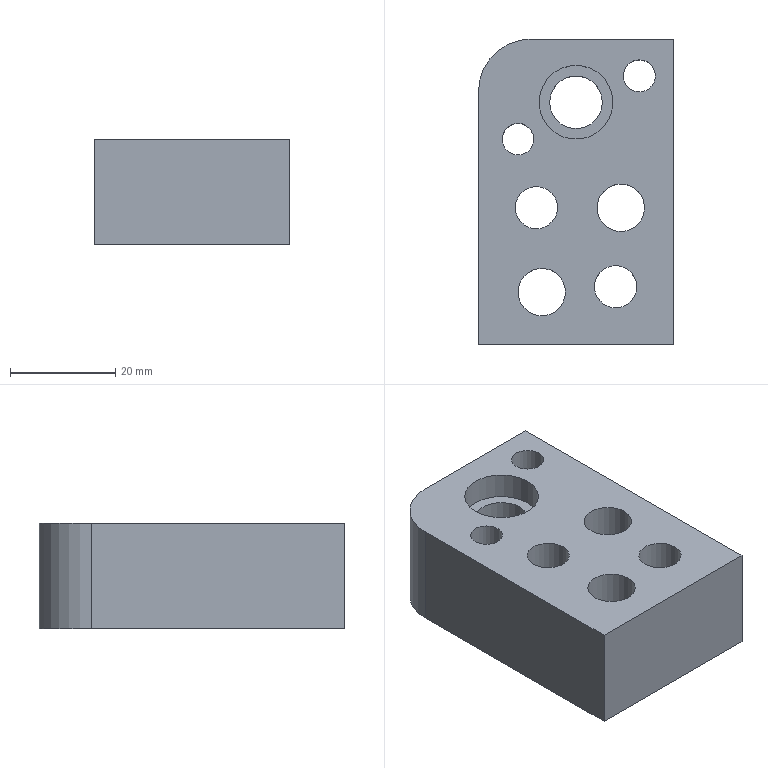Part | STEP file | 414_id2066_x_t | 1 solid | 24 faces | box 37 x 58 x 20 mm | volume 32466 mm3 | cylinder 13 | plane 11 | commonest cylinder face diameters 10 x3 14 x3 8 x2 9 x2 6 x1 6.1 x1